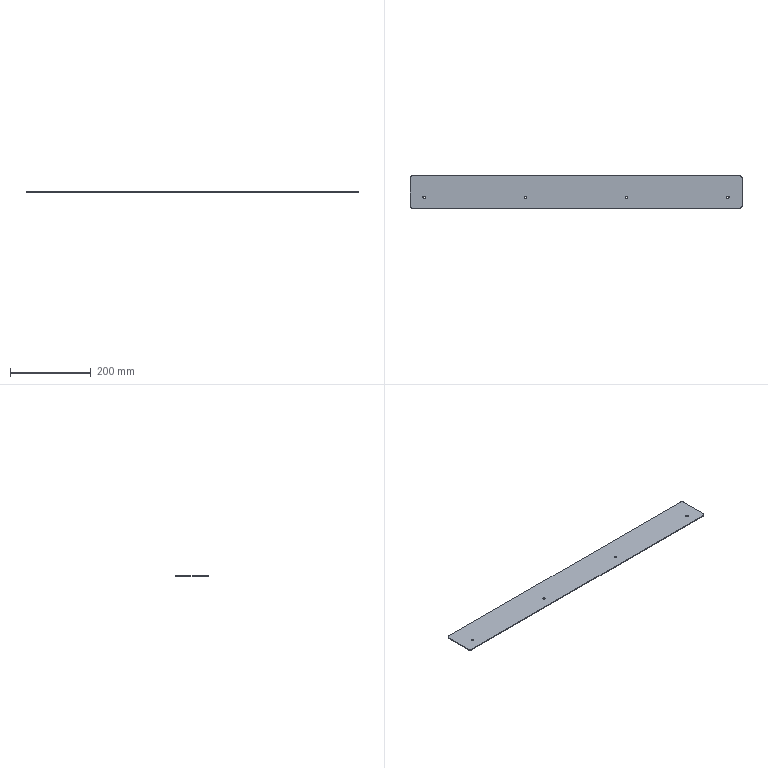Part | STEP file | 1 solid | 18 faces | box 820 x 80 x 2 mm | volume 130931 mm3 | cylinder 12 | plane 6 | commonest cylinder face diameters 6 x8 10 x4
STEP:
#1=CARTESIAN_POINT('',(0.,0.,0.));
#2=DIRECTION('',(0.,0.,1.));
#3=DIRECTION('',(1.,0.,0.));
#4=AXIS2_PLACEMENT_3D('',#1,#2,#3);
#5=CARTESIAN_POINT('',(-128.,-13.,2.));
#6=VERTEX_POINT('',#5);
#7=CARTESIAN_POINT('',(-128.,-13.,0.));
#8=VERTEX_POINT('',#7);
#9=CARTESIAN_POINT('',(-128.,-13.,0.));
#10=DIRECTION('',(0.,0.,-1.));
#11=VECTOR('',#10,1.);
#12=LINE('',#9,#11);
#13=CARTESIAN_POINT('',(-125.,-13.,0.));
#14=DIRECTION('',(0.,0.,-1.));
#15=DIRECTION('',(-1.,0.,0.));
#16=AXIS2_PLACEMENT_3D('',#13,#14,#15);
#17=CYLINDRICAL_SURFACE('',#16,3.);
#18=CARTESIAN_POINT('',(6.283,0.));
#19=DIRECTION('',(0.,1.));
#20=VECTOR('',#19,1.);
#21=LINE('',#18,#20);
#22=(GEOMETRIC_REPRESENTATION_CONTEXT(2)PARAMETRIC_REPRESENTATION_CONTEXT()REPRESENTATION_CONTEXT('',''));
#23=DEFINITIONAL_REPRESENTATION('',(#21),#22);
#24=PCURVE('',#17,#23);
#25=CARTESIAN_POINT('',(-125.,-13.,0.));
#26=DIRECTION('',(0.,0.,-1.));
#27=DIRECTION('',(-1.,0.,0.));
#28=AXIS2_PLACEMENT_3D('',#25,#26,#27);
#29=CYLINDRICAL_SURFACE('',#28,3.);
#30=CARTESIAN_POINT('',(0.,0.));
#31=DIRECTION('',(0.,1.));
#32=VECTOR('',#31,1.);
#33=LINE('',#30,#32);
#34=(GEOMETRIC_REPRESENTATION_CONTEXT(2)PARAMETRIC_REPRESENTATION_CONTEXT()REPRESENTATION_CONTEXT('',''));
#35=DEFINITIONAL_REPRESENTATION('',(#33),#34);
#36=PCURVE('',#29,#35);
#37=SURFACE_CURVE('',#12,(#24,#36),.PCURVE_S1.);
#38=EDGE_CURVE('',#6,#8,#37,.T.);
#39=ORIENTED_EDGE('',*,*,#38,.T.);
#40=CARTESIAN_POINT('',(-122.,-13.,0.));
#41=VERTEX_POINT('',#40);
#42=CARTESIAN_POINT('',(-125.,-13.,0.));
#43=DIRECTION('',(0.,0.,1.));
#44=DIRECTION('',(-1.,0.,0.));
#45=AXIS2_PLACEMENT_3D('',#42,#43,#44);
#46=CIRCLE('',#45,3.);
#47=CARTESIAN_POINT('',(6.283,0.));
#48=DIRECTION('',(-1.,0.));
#49=VECTOR('',#48,1.);
#50=LINE('',#47,#49);
#51=(GEOMETRIC_REPRESENTATION_CONTEXT(2)PARAMETRIC_REPRESENTATION_CONTEXT()REPRESENTATION_CONTEXT('',''));
#52=DEFINITIONAL_REPRESENTATION('',(#50),#51);
#53=PCURVE('',#17,#52);
#54=CARTESIAN_POINT('',(410.,-40.,0.));
#55=DIRECTION('',(0.,0.,1.));
#56=DIRECTION('',(1.,0.,0.));
#57=AXIS2_PLACEMENT_3D('',#54,#55,#56);
#58=PLANE('',#57);
#59=CARTESIAN_POINT('',(-535.,27.));
#60=DIRECTION('',(-1.,0.));
#61=AXIS2_PLACEMENT_2D('',#59,#60);
#62=CIRCLE('',#61,3.);
#63=(GEOMETRIC_REPRESENTATION_CONTEXT(2)PARAMETRIC_REPRESENTATION_CONTEXT()REPRESENTATION_CONTEXT('',''));
#64=DEFINITIONAL_REPRESENTATION('',(#62),#63);
#65=PCURVE('',#58,#64);
#66=SURFACE_CURVE('',#46,(#53,#65),.PCURVE_S1.);
#67=EDGE_CURVE('',#8,#41,#66,.T.);
#68=ORIENTED_EDGE('',*,*,#67,.T.);
#69=CARTESIAN_POINT('',(-122.,-13.,2.));
#70=VERTEX_POINT('',#69);
#71=CARTESIAN_POINT('',(-122.,-13.,0.));
#72=DIRECTION('',(0.,0.,-1.));
#73=VECTOR('',#72,1.);
#74=LINE('',#71,#73);
#75=CARTESIAN_POINT('',(3.142,0.));
#76=DIRECTION('',(0.,1.));
#77=VECTOR('',#76,1.);
#78=LINE('',#75,#77);
#79=(GEOMETRIC_REPRESENTATION_CONTEXT(2)PARAMETRIC_REPRESENTATION_CONTEXT()REPRESENTATION_CONTEXT('',''));
#80=DEFINITIONAL_REPRESENTATION('',(#78),#79);
#81=PCURVE('',#17,#80);
#82=CARTESIAN_POINT('',(3.142,0.));
#83=DIRECTION('',(0.,1.));
#84=VECTOR('',#83,1.);
#85=LINE('',#82,#84);
#86=(GEOMETRIC_REPRESENTATION_CONTEXT(2)PARAMETRIC_REPRESENTATION_CONTEXT()REPRESENTATION_CONTEXT('',''));
#87=DEFINITIONAL_REPRESENTATION('',(#85),#86);
#88=PCURVE('',#29,#87);
#89=SURFACE_CURVE('',#74,(#81,#88),.PCURVE_S1.);
#90=EDGE_CURVE('',#70,#41,#89,.T.);
#91=ORIENTED_EDGE('',*,*,#90,.F.);
#92=CARTESIAN_POINT('',(-125.,-13.,2.));
#93=DIRECTION('',(0.,0.,-1.));
#94=DIRECTION('',(-1.,0.,0.));
#95=AXIS2_PLACEMENT_3D('',#92,#93,#94);
#96=CIRCLE('',#95,3.);
#97=CARTESIAN_POINT('',(0.,-2.));
#98=DIRECTION('',(1.,0.));
#99=VECTOR('',#98,1.);
#100=LINE('',#97,#99);
#101=(GEOMETRIC_REPRESENTATION_CONTEXT(2)PARAMETRIC_REPRESENTATION_CONTEXT()REPRESENTATION_CONTEXT('',''));
#102=DEFINITIONAL_REPRESENTATION('',(#100),#101);
#103=PCURVE('',#17,#102);
#104=CARTESIAN_POINT('',(410.,-40.,2.));
#105=DIRECTION('',(0.,0.,1.));
#106=DIRECTION('',(1.,0.,0.));
#107=AXIS2_PLACEMENT_3D('',#104,#105,#106);
#108=PLANE('',#107);
#109=CARTESIAN_POINT('',(-538.,27.));
#110=CARTESIAN_POINT('',(-538.,32.196));
#111=CARTESIAN_POINT('',(-533.5,29.598));
#112=CARTESIAN_POINT('',(-529.,27.));
#113=CARTESIAN_POINT('',(-533.5,24.402));
#114=CARTESIAN_POINT('',(-538.,21.804));
#115=CARTESIAN_POINT('',(-538.,27.));
#116=(BOUNDED_CURVE()B_SPLINE_CURVE(2,(#109,#110,#111,#112,#113,#114,#115),.UNSPECIFIED.,.T.,.F.)B_SPLINE_CURVE_WITH_KNOTS((1,2,2,2,2,1),(-2.094,0.,2.094,4.189,6.283,8.378),.UNSPECIFIED.)CURVE()GEOMETRIC_REPRESENTATION_ITEM()RATIONAL_B_SPLINE_CURVE((1.,0.5,1.,0.5,1.,0.5,1.))REPRESENTATION_ITEM(''));
#117=(GEOMETRIC_REPRESENTATION_CONTEXT(2)PARAMETRIC_REPRESENTATION_CONTEXT()REPRESENTATION_CONTEXT('',''));
#118=DEFINITIONAL_REPRESENTATION('',(#116),#117);
#119=PCURVE('',#108,#118);
#120=SURFACE_CURVE('',#96,(#103,#119),.PCURVE_S1.);
#121=EDGE_CURVE('',#70,#6,#120,.T.);
#122=ORIENTED_EDGE('',*,*,#121,.T.);
#123=EDGE_LOOP('',(#39,#68,#91,#122));
#124=FACE_BOUND('',#123,.F.);
#125=ADVANCED_FACE('',(#124),#17,.F.);
#126=CARTESIAN_POINT('',(-378.,-13.,2.));
#127=VERTEX_POINT('',#126);
#128=CARTESIAN_POINT('',(-378.,-13.,0.));
#129=VERTEX_POINT('',#128);
#130=CARTESIAN_POINT('',(-378.,-13.,0.));
#131=DIRECTION('',(0.,0.,-1.));
#132=VECTOR('',#131,1.);
#133=LINE('',#130,#132);
#134=CARTESIAN_POINT('',(-375.,-13.,0.));
#135=DIRECTION('',(0.,0.,-1.));
#136=DIRECTION('',(-1.,0.,0.));
#137=AXIS2_PLACEMENT_3D('',#134,#135,#136);
#138=CYLINDRICAL_SURFACE('',#137,3.);
#139=CARTESIAN_POINT('',(6.283,0.));
#140=DIRECTION('',(0.,1.));
#141=VECTOR('',#140,1.);
#142=LINE('',#139,#141);
#143=(GEOMETRIC_REPRESENTATION_CONTEXT(2)PARAMETRIC_REPRESENTATION_CONTEXT()REPRESENTATION_CONTEXT('',''));
#144=DEFINITIONAL_REPRESENTATION('',(#142),#143);
#145=PCURVE('',#138,#144);
#146=CARTESIAN_POINT('',(-375.,-13.,0.));
#147=DIRECTION('',(0.,0.,-1.));
#148=DIRECTION('',(-1.,0.,0.));
#149=AXIS2_PLACEMENT_3D('',#146,#147,#148);
#150=CYLINDRICAL_SURFACE('',#149,3.);
#151=CARTESIAN_POINT('',(0.,0.));
#152=DIRECTION('',(0.,1.));
#153=VECTOR('',#152,1.);
#154=LINE('',#151,#153);
#155=(GEOMETRIC_REPRESENTATION_CONTEXT(2)PARAMETRIC_REPRESENTATION_CONTEXT()REPRESENTATION_CONTEXT('',''));
#156=DEFINITIONAL_REPRESENTATION('',(#154),#155);
#157=PCURVE('',#150,#156);
#158=SURFACE_CURVE('',#133,(#145,#157),.PCURVE_S1.);
#159=EDGE_CURVE('',#127,#129,#158,.T.);
#160=ORIENTED_EDGE('',*,*,#159,.T.);
#161=CARTESIAN_POINT('',(-372.,-13.,0.));
#162=VERTEX_POINT('',#161);
#163=CARTESIAN_POINT('',(-375.,-13.,0.));
#164=DIRECTION('',(0.,0.,1.));
#165=DIRECTION('',(-1.,0.,0.));
#166=AXIS2_PLACEMENT_3D('',#163,#164,#165);
#167=CIRCLE('',#166,3.);
#168=CARTESIAN_POINT('',(6.283,0.));
#169=DIRECTION('',(-1.,0.));
#170=VECTOR('',#169,1.);
#171=LINE('',#168,#170);
#172=(GEOMETRIC_REPRESENTATION_CONTEXT(2)PARAMETRIC_REPRESENTATION_CONTEXT()REPRESENTATION_CONTEXT('',''));
#173=DEFINITIONAL_REPRESENTATION('',(#171),#172);
#174=PCURVE('',#138,#173);
#175=CARTESIAN_POINT('',(-785.,27.));
#176=DIRECTION('',(-1.,0.));
#177=AXIS2_PLACEMENT_2D('',#175,#176);
#178=CIRCLE('',#177,3.);
#179=(GEOMETRIC_REPRESENTATION_CONTEXT(2)PARAMETRIC_REPRESENTATION_CONTEXT()REPRESENTATION_CONTEXT('',''));
#180=DEFINITIONAL_REPRESENTATION('',(#178),#179);
#181=PCURVE('',#58,#180);
#182=SURFACE_CURVE('',#167,(#174,#181),.PCURVE_S1.);
#183=EDGE_CURVE('',#129,#162,#182,.T.);
#184=ORIENTED_EDGE('',*,*,#183,.T.);
#185=CARTESIAN_POINT('',(-372.,-13.,2.));
#186=VERTEX_POINT('',#185);
#187=CARTESIAN_POINT('',(-372.,-13.,0.));
#188=DIRECTION('',(0.,0.,-1.));
#189=VECTOR('',#188,1.);
#190=LINE('',#187,#189);
#191=CARTESIAN_POINT('',(3.142,0.));
#192=DIRECTION('',(0.,1.));
#193=VECTOR('',#192,1.);
#194=LINE('',#191,#193);
#195=(GEOMETRIC_REPRESENTATION_CONTEXT(2)PARAMETRIC_REPRESENTATION_CONTEXT()REPRESENTATION_CONTEXT('',''));
#196=DEFINITIONAL_REPRESENTATION('',(#194),#195);
#197=PCURVE('',#138,#196);
#198=CARTESIAN_POINT('',(3.142,0.));
#199=DIRECTION('',(0.,1.));
#200=VECTOR('',#199,1.);
#201=LINE('',#198,#200);
#202=(GEOMETRIC_REPRESENTATION_CONTEXT(2)PARAMETRIC_REPRESENTATION_CONTEXT()REPRESENTATION_CONTEXT('',''));
#203=DEFINITIONAL_REPRESENTATION('',(#201),#202);
#204=PCURVE('',#150,#203);
#205=SURFACE_CURVE('',#190,(#197,#204),.PCURVE_S1.);
#206=EDGE_CURVE('',#186,#162,#205,.T.);
#207=ORIENTED_EDGE('',*,*,#206,.F.);
#208=CARTESIAN_POINT('',(-375.,-13.,2.));
#209=DIRECTION('',(0.,0.,-1.));
#210=DIRECTION('',(-1.,0.,0.));
#211=AXIS2_PLACEMENT_3D('',#208,#209,#210);
#212=CIRCLE('',#211,3.);
#213=CARTESIAN_POINT('',(0.,-2.));
#214=DIRECTION('',(1.,0.));
#215=VECTOR('',#214,1.);
#216=LINE('',#213,#215);
#217=(GEOMETRIC_REPRESENTATION_CONTEXT(2)PARAMETRIC_REPRESENTATION_CONTEXT()REPRESENTATION_CONTEXT('',''));
#218=DEFINITIONAL_REPRESENTATION('',(#216),#217);
#219=PCURVE('',#138,#218);
#220=CARTESIAN_POINT('',(-788.,27.));
#221=CARTESIAN_POINT('',(-788.,32.196));
#222=CARTESIAN_POINT('',(-783.5,29.598));
#223=CARTESIAN_POINT('',(-779.,27.));
#224=CARTESIAN_POINT('',(-783.5,24.402));
#225=CARTESIAN_POINT('',(-788.,21.804));
#226=CARTESIAN_POINT('',(-788.,27.));
#227=(BOUNDED_CURVE()B_SPLINE_CURVE(2,(#220,#221,#222,#223,#224,#225,#226),.UNSPECIFIED.,.T.,.F.)B_SPLINE_CURVE_WITH_KNOTS((1,2,2,2,2,1),(-2.094,0.,2.094,4.189,6.283,8.378),.UNSPECIFIED.)CURVE()GEOMETRIC_REPRESENTATION_ITEM()RATIONAL_B_SPLINE_CURVE((1.,0.5,1.,0.5,1.,0.5,1.))REPRESENTATION_ITEM(''));
#228=(GEOMETRIC_REPRESENTATION_CONTEXT(2)PARAMETRIC_REPRESENTATION_CONTEXT()REPRESENTATION_CONTEXT('',''));
#229=DEFINITIONAL_REPRESENTATION('',(#227),#228);
#230=PCURVE('',#108,#229);
#231=SURFACE_CURVE('',#212,(#219,#230),.PCURVE_S1.);
#232=EDGE_CURVE('',#186,#127,#231,.T.);
#233=ORIENTED_EDGE('',*,*,#232,.T.);
#234=EDGE_LOOP('',(#160,#184,#207,#233));
#235=FACE_BOUND('',#234,.F.);
#236=ADVANCED_FACE('',(#235),#138,.F.);
#237=CARTESIAN_POINT('',(122.,-13.,2.));
#238=VERTEX_POINT('',#237);
#239=CARTESIAN_POINT('',(122.,-13.,0.));
#240=VERTEX_POINT('',#239);
#241=CARTESIAN_POINT('',(122.,-13.,0.));
#242=DIRECTION('',(0.,0.,-1.));
#243=VECTOR('',#242,1.);
#244=LINE('',#241,#243);
#245=CARTESIAN_POINT('',(125.,-13.,0.));
#246=DIRECTION('',(0.,0.,-1.));
#247=DIRECTION('',(-1.,0.,0.));
#248=AXIS2_PLACEMENT_3D('',#245,#246,#247);
#249=CYLINDRICAL_SURFACE('',#248,3.);
#250=CARTESIAN_POINT('',(6.283,0.));
#251=DIRECTION('',(0.,1.));
#252=VECTOR('',#251,1.);
#253=LINE('',#250,#252);
#254=(GEOMETRIC_REPRESENTATION_CONTEXT(2)PARAMETRIC_REPRESENTATION_CONTEXT()REPRESENTATION_CONTEXT('',''));
#255=DEFINITIONAL_REPRESENTATION('',(#253),#254);
#256=PCURVE('',#249,#255);
#257=CARTESIAN_POINT('',(125.,-13.,0.));
#258=DIRECTION('',(0.,0.,-1.));
#259=DIRECTION('',(-1.,0.,0.));
#260=AXIS2_PLACEMENT_3D('',#257,#258,#259);
#261=CYLINDRICAL_SURFACE('',#260,3.);
#262=CARTESIAN_POINT('',(0.,0.));
#263=DIRECTION('',(0.,1.));
#264=VECTOR('',#263,1.);
#265=LINE('',#262,#264);
#266=(GEOMETRIC_REPRESENTATION_CONTEXT(2)PARAMETRIC_REPRESENTATION_CONTEXT()REPRESENTATION_CONTEXT('',''));
#267=DEFINITIONAL_REPRESENTATION('',(#265),#266);
#268=PCURVE('',#261,#267);
#269=SURFACE_CURVE('',#244,(#256,#268),.PCURVE_S1.);
#270=EDGE_CURVE('',#238,#240,#269,.T.);
#271=ORIENTED_EDGE('',*,*,#270,.T.);
#272=CARTESIAN_POINT('',(128.,-13.,0.));
#273=VERTEX_POINT('',#272);
#274=CARTESIAN_POINT('',(125.,-13.,0.));
#275=DIRECTION('',(0.,0.,1.));
#276=DIRECTION('',(-1.,0.,0.));
#277=AXIS2_PLACEMENT_3D('',#274,#275,#276);
#278=CIRCLE('',#277,3.);
#279=CARTESIAN_POINT('',(6.283,0.));
#280=DIRECTION('',(-1.,0.));
#281=VECTOR('',#280,1.);
#282=LINE('',#279,#281);
#283=(GEOMETRIC_REPRESENTATION_CONTEXT(2)PARAMETRIC_REPRESENTATION_CONTEXT()REPRESENTATION_CONTEXT('',''));
#284=DEFINITIONAL_REPRESENTATION('',(#282),#283);
#285=PCURVE('',#249,#284);
#286=CARTESIAN_POINT('',(-285.,27.));
#287=DIRECTION('',(-1.,0.));
#288=AXIS2_PLACEMENT_2D('',#286,#287);
#289=CIRCLE('',#288,3.);
#290=(GEOMETRIC_REPRESENTATION_CONTEXT(2)PARAMETRIC_REPRESENTATION_CONTEXT()REPRESENTATION_CONTEXT('',''));
#291=DEFINITIONAL_REPRESENTATION('',(#289),#290);
#292=PCURVE('',#58,#291);
#293=SURFACE_CURVE('',#278,(#285,#292),.PCURVE_S1.);
#294=EDGE_CURVE('',#240,#273,#293,.T.);
#295=ORIENTED_EDGE('',*,*,#294,.T.);
#296=CARTESIAN_POINT('',(128.,-13.,2.));
#297=VERTEX_POINT('',#296);
#298=CARTESIAN_POINT('',(128.,-13.,0.));
#299=DIRECTION('',(0.,0.,-1.));
#300=VECTOR('',#299,1.);
#301=LINE('',#298,#300);
#302=CARTESIAN_POINT('',(3.142,0.));
#303=DIRECTION('',(0.,1.));
#304=VECTOR('',#303,1.);
#305=LINE('',#302,#304);
#306=(GEOMETRIC_REPRESENTATION_CONTEXT(2)PARAMETRIC_REPRESENTATION_CONTEXT()REPRESENTATION_CONTEXT('',''));
#307=DEFINITIONAL_REPRESENTATION('',(#305),#306);
#308=PCURVE('',#249,#307);
#309=CARTESIAN_POINT('',(3.142,0.));
#310=DIRECTION('',(0.,1.));
#311=VECTOR('',#310,1.);
#312=LINE('',#309,#311);
#313=(GEOMETRIC_REPRESENTATION_CONTEXT(2)PARAMETRIC_REPRESENTATION_CONTEXT()REPRESENTATION_CONTEXT('',''));
#314=DEFINITIONAL_REPRESENTATION('',(#312),#313);
#315=PCURVE('',#261,#314);
#316=SURFACE_CURVE('',#301,(#308,#315),.PCURVE_S1.);
#317=EDGE_CURVE('',#297,#273,#316,.T.);
#318=ORIENTED_EDGE('',*,*,#317,.F.);
#319=CARTESIAN_POINT('',(125.,-13.,2.));
#320=DIRECTION('',(0.,0.,-1.));
#321=DIRECTION('',(-1.,0.,0.));
#322=AXIS2_PLACEMENT_3D('',#319,#320,#321);
#323=CIRCLE('',#322,3.);
#324=CARTESIAN_POINT('',(0.,-2.));
#325=DIRECTION('',(1.,0.));
#326=VECTOR('',#325,1.);
#327=LINE('',#324,#326);
#328=(GEOMETRIC_REPRESENTATION_CONTEXT(2)PARAMETRIC_REPRESENTATION_CONTEXT()REPRESENTATION_CONTEXT('',''));
#329=DEFINITIONAL_REPRESENTATION('',(#327),#328);
#330=PCURVE('',#249,#329);
#331=CARTESIAN_POINT('',(-288.,27.));
#332=CARTESIAN_POINT('',(-288.,32.196));
#333=CARTESIAN_POINT('',(-283.5,29.598));
#334=CARTESIAN_POINT('',(-279.,27.));
#335=CARTESIAN_POINT('',(-283.5,24.402));
#336=CARTESIAN_POINT('',(-288.,21.804));
#337=CARTESIAN_POINT('',(-288.,27.));
#338=(BOUNDED_CURVE()B_SPLINE_CURVE(2,(#331,#332,#333,#334,#335,#336,#337),.UNSPECIFIED.,.T.,.F.)B_SPLINE_CURVE_WITH_KNOTS((1,2,2,2,2,1),(-2.094,0.,2.094,4.189,6.283,8.378),.UNSPECIFIED.)CURVE()GEOMETRIC_REPRESENTATION_ITEM()RATIONAL_B_SPLINE_CURVE((1.,0.5,1.,0.5,1.,0.5,1.))REPRESENTATION_ITEM(''));
#339=(GEOMETRIC_REPRESENTATION_CONTEXT(2)PARAMETRIC_REPRESENTATION_CONTEXT()REPRESENTATION_CONTEXT('',''));
#340=DEFINITIONAL_REPRESENTATION('',(#338),#339);
#341=PCURVE('',#108,#340);
#342=SURFACE_CURVE('',#323,(#330,#341),.PCURVE_S1.);
#343=EDGE_CURVE('',#297,#238,#342,.T.);
#344=ORIENTED_EDGE('',*,*,#343,.T.);
#345=EDGE_LOOP('',(#271,#295,#318,#344));
#346=FACE_BOUND('',#345,.F.);
#347=ADVANCED_FACE('',(#346),#249,.F.);
#348=CARTESIAN_POINT('',(372.,-13.,2.));
#349=VERTEX_POINT('',#348);
#350=CARTESIAN_POINT('',(372.,-13.,0.));
#351=VERTEX_POINT('',#350);
#352=CARTESIAN_POINT('',(372.,-13.,0.));
#353=DIRECTION('',(0.,0.,-1.));
#354=VECTOR('',#353,1.);
#355=LINE('',#352,#354);
#356=CARTESIAN_POINT('',(375.,-13.,0.));
#357=DIRECTION('',(0.,0.,-1.));
#358=DIRECTION('',(-1.,0.,0.));
#359=AXIS2_PLACEMENT_3D('',#356,#357,#358);
#360=CYLINDRICAL_SURFACE('',#359,3.);
#361=CARTESIAN_POINT('',(6.283,0.));
#362=DIRECTION('',(0.,1.));
#363=VECTOR('',#362,1.);
#364=LINE('',#361,#363);
#365=(GEOMETRIC_REPRESENTATION_CONTEXT(2)PARAMETRIC_REPRESENTATION_CONTEXT()REPRESENTATION_CONTEXT('',''));
#366=DEFINITIONAL_REPRESENTATION('',(#364),#365);
#367=PCURVE('',#360,#366);
#368=CARTESIAN_POINT('',(375.,-13.,0.));
#369=DIRECTION('',(0.,0.,-1.));
#370=DIRECTION('',(-1.,0.,0.));
#371=AXIS2_PLACEMENT_3D('',#368,#369,#370);
#372=CYLINDRICAL_SURFACE('',#371,3.);
#373=CARTESIAN_POINT('',(0.,0.));
#374=DIRECTION('',(0.,1.));
#375=VECTOR('',#374,1.);
#376=LINE('',#373,#375);
#377=(GEOMETRIC_REPRESENTATION_CONTEXT(2)PARAMETRIC_REPRESENTATION_CONTEXT()REPRESENTATION_CONTEXT('',''));
#378=DEFINITIONAL_REPRESENTATION('',(#376),#377);
#379=PCURVE('',#372,#378);
#380=SURFACE_CURVE('',#355,(#367,#379),.PCURVE_S1.);
#381=EDGE_CURVE('',#349,#351,#380,.T.);
#382=ORIENTED_EDGE('',*,*,#381,.T.);
#383=CARTESIAN_POINT('',(378.,-13.,0.));
#384=VERTEX_POINT('',#383);
#385=CARTESIAN_POINT('',(375.,-13.,0.));
#386=DIRECTION('',(0.,0.,1.));
#387=DIRECTION('',(-1.,0.,0.));
#388=AXIS2_PLACEMENT_3D('',#385,#386,#387);
#389=CIRCLE('',#388,3.);
#390=CARTESIAN_POINT('',(6.283,0.));
#391=DIRECTION('',(-1.,0.));
#392=VECTOR('',#391,1.);
#393=LINE('',#390,#392);
#394=(GEOMETRIC_REPRESENTATION_CONTEXT(2)PARAMETRIC_REPRESENTATION_CONTEXT()REPRESENTATION_CONTEXT('',''));
#395=DEFINITIONAL_REPRESENTATION('',(#393),#394);
#396=PCURVE('',#360,#395);
#397=CARTESIAN_POINT('',(-35.,27.));
#398=DIRECTION('',(-1.,0.));
#399=AXIS2_PLACEMENT_2D('',#397,#398);
#400=CIRCLE('',#399,3.);
#401=(GEOMETRIC_REPRESENTATION_CONTEXT(2)PARAMETRIC_REPRESENTATION_CONTEXT()REPRESENTATION_CONTEXT('',''));
#402=DEFINITIONAL_REPRESENTATION('',(#400),#401);
#403=PCURVE('',#58,#402);
#404=SURFACE_CURVE('',#389,(#396,#403),.PCURVE_S1.);
#405=EDGE_CURVE('',#351,#384,#404,.T.);
#406=ORIENTED_EDGE('',*,*,#405,.T.);
#407=CARTESIAN_POINT('',(378.,-13.,2.));
#408=VERTEX_POINT('',#407);
#409=CARTESIAN_POINT('',(378.,-13.,0.));
#410=DIRECTION('',(0.,0.,-1.));
#411=VECTOR('',#410,1.);
#412=LINE('',#409,#411);
#413=CARTESIAN_POINT('',(3.142,0.));
#414=DIRECTION('',(0.,1.));
#415=VECTOR('',#414,1.);
#416=LINE('',#413,#415);
#417=(GEOMETRIC_REPRESENTATION_CONTEXT(2)PARAMETRIC_REPRESENTATION_CONTEXT()REPRESENTATION_CONTEXT('',''));
#418=DEFINITIONAL_REPRESENTATION('',(#416),#417);
#419=PCURVE('',#360,#418);
#420=CARTESIAN_POINT('',(3.142,0.));
#421=DIRECTION('',(0.,1.));
#422=VECTOR('',#421,1.);
#423=LINE('',#420,#422);
#424=(GEOMETRIC_REPRESENTATION_CONTEXT(2)PARAMETRIC_REPRESENTATION_CONTEXT()REPRESENTATION_CONTEXT('',''));
#425=DEFINITIONAL_REPRESENTATION('',(#423),#424);
#426=PCURVE('',#372,#425);
#427=SURFACE_CURVE('',#412,(#419,#426),.PCURVE_S1.);
#428=EDGE_CURVE('',#408,#384,#427,.T.);
#429=ORIENTED_EDGE('',*,*,#428,.F.);
#430=CARTESIAN_POINT('',(375.,-13.,2.));
#431=DIRECTION('',(0.,0.,-1.));
#432=DIRECTION('',(-1.,0.,0.));
#433=AXIS2_PLACEMENT_3D('',#430,#431,#432);
#434=CIRCLE('',#433,3.);
#435=CARTESIAN_POINT('',(0.,-2.));
#436=DIRECTION('',(1.,0.));
#437=VECTOR('',#436,1.);
#438=LINE('',#435,#437);
#439=(GEOMETRIC_REPRESENTATION_CONTEXT(2)PARAMETRIC_REPRESENTATION_CONTEXT()REPRESENTATION_CONTEXT('',''));
#440=DEFINITIONAL_REPRESENTATION('',(#438),#439);
#441=PCURVE('',#360,#440);
#442=CARTESIAN_POINT('',(-38.,27.));
#443=CARTESIAN_POINT('',(-38.,32.196));
#444=CARTESIAN_POINT('',(-33.5,29.598));
#445=CARTESIAN_POINT('',(-29.,27.));
#446=CARTESIAN_POINT('',(-33.5,24.402));
#447=CARTESIAN_POINT('',(-38.,21.804));
#448=CARTESIAN_POINT('',(-38.,27.));
#449=(BOUNDED_CURVE()B_SPLINE_CURVE(2,(#442,#443,#444,#445,#446,#447,#448),.UNSPECIFIED.,.T.,.F.)B_SPLINE_CURVE_WITH_KNOTS((1,2,2,2,2,1),(-2.094,0.,2.094,4.189,6.283,8.378),.UNSPECIFIED.)CURVE()GEOMETRIC_REPRESENTATION_ITEM()RATIONAL_B_SPLINE_CURVE((1.,0.5,1.,0.5,1.,0.5,1.))REPRESENTATION_ITEM(''));
#450=(GEOMETRIC_REPRESENTATION_CONTEXT(2)PARAMETRIC_REPRESENTATION_CONTEXT()REPRESENTATION_CONTEXT('',''));
#451=DEFINITIONAL_REPRESENTATION('',(#449),#450);
#452=PCURVE('',#108,#451);
#453=SURFACE_CURVE('',#434,(#441,#452),.PCURVE_S1.);
#454=EDGE_CURVE('',#408,#349,#453,.T.);
#455=ORIENTED_EDGE('',*,*,#454,.T.);
#456=EDGE_LOOP('',(#382,#406,#429,#455));
#457=FACE_BOUND('',#456,.F.);
#458=ADVANCED_FACE('',(#457),#360,.F.);
#459=CARTESIAN_POINT('',(-125.,-13.,2.));
#460=DIRECTION('',(0.,0.,-1.));
#461=DIRECTION('',(-1.,0.,0.));
#462=AXIS2_PLACEMENT_3D('',#459,#460,#461);
#463=CIRCLE('',#462,3.);
#464=CARTESIAN_POINT('',(-538.,27.));
#465=CARTESIAN_POINT('',(-538.,32.196));
#466=CARTESIAN_POINT('',(-533.5,29.598));
#467=CARTESIAN_POINT('',(-529.,27.));
#468=CARTESIAN_POINT('',(-533.5,24.402));
#469=CARTESIAN_POINT('',(-538.,21.804));
#470=CARTESIAN_POINT('',(-538.,27.));
#471=(BOUNDED_CURVE()B_SPLINE_CURVE(2,(#464,#465,#466,#467,#468,#469,#470),.UNSPECIFIED.,.T.,.F.)B_SPLINE_CURVE_WITH_KNOTS((1,2,2,2,2,1),(-2.094,0.,2.094,4.189,6.283,8.378),.UNSPECIFIED.)CURVE()GEOMETRIC_REPRESENTATION_ITEM()RATIONAL_B_SPLINE_CURVE((1.,0.5,1.,0.5,1.,0.5,1.))REPRESENTATION_ITEM(''));
#472=(GEOMETRIC_REPRESENTATION_CONTEXT(2)PARAMETRIC_REPRESENTATION_CONTEXT()REPRESENTATION_CONTEXT('',''));
#473=DEFINITIONAL_REPRESENTATION('',(#471),#472);
#474=PCURVE('',#108,#473);
#475=CARTESIAN_POINT('',(0.,-2.));
#476=DIRECTION('',(1.,0.));
#477=VECTOR('',#476,1.);
#478=LINE('',#475,#477);
#479=(GEOMETRIC_REPRESENTATION_CONTEXT(2)PARAMETRIC_REPRESENTATION_CONTEXT()REPRESENTATION_CONTEXT('',''));
#480=DEFINITIONAL_REPRESENTATION('',(#478),#479);
#481=PCURVE('',#29,#480);
#482=SURFACE_CURVE('',#463,(#474,#481),.PCURVE_S1.);
#483=EDGE_CURVE('',#6,#70,#482,.T.);
#484=ORIENTED_EDGE('',*,*,#483,.T.);
#485=ORIENTED_EDGE('',*,*,#121,.T.);
#486=EDGE_LOOP('',(#484,#485));
#487=FACE_BOUND('',#486,.T.);
#488=CARTESIAN_POINT('',(-375.,-13.,2.));
#489=DIRECTION('',(0.,0.,-1.));
#490=DIRECTION('',(-1.,0.,0.));
#491=AXIS2_PLACEMENT_3D('',#488,#489,#490);
#492=CIRCLE('',#491,3.);
#493=CARTESIAN_POINT('',(-788.,27.));
#494=CARTESIAN_POINT('',(-788.,32.196));
#495=CARTESIAN_POINT('',(-783.5,29.598));
#496=CARTESIAN_POINT('',(-779.,27.));
#497=CARTESIAN_POINT('',(-783.5,24.402));
#498=CARTESIAN_POINT('',(-788.,21.804));
#499=CARTESIAN_POINT('',(-788.,27.));
#500=(BOUNDED_CURVE()B_SPLINE_CURVE(2,(#493,#494,#495,#496,#497,#498,#499),.UNSPECIFIED.,.T.,.F.)B_SPLINE_CURVE_WITH_KNOTS((1,2,2,2,2,1),(-2.094,0.,2.094,4.189,6.283,8.378),.UNSPECIFIED.)CURVE()GEOMETRIC_REPRESENTATION_ITEM()RATIONAL_B_SPLINE_CURVE((1.,0.5,1.,0.5,1.,0.5,1.))REPRESENTATION_ITEM(''));
#501=(GEOMETRIC_REPRESENTATION_CONTEXT(2)PARAMETRIC_REPRESENTATION_CONTEXT()REPRESENTATION_CONTEXT('',''));
#502=DEFINITIONAL_REPRESENTATION('',(#500),#501);
#503=PCURVE('',#108,#502);
#504=CARTESIAN_POINT('',(0.,-2.));
#505=DIRECTION('',(1.,0.));
#506=VECTOR('',#505,1.);
#507=LINE('',#504,#506);
#508=(GEOMETRIC_REPRESENTATION_CONTEXT(2)PARAMETRIC_REPRESENTATION_CONTEXT()REPRESENTATION_CONTEXT('',''));
#509=DEFINITIONAL_REPRESENTATION('',(#507),#508);
#510=PCURVE('',#150,#509);
#511=SURFACE_CURVE('',#492,(#503,#510),.PCURVE_S1.);
#512=EDGE_CURVE('',#127,#186,#511,.T.);
#513=ORIENTED_EDGE('',*,*,#512,.T.);
#514=ORIENTED_EDGE('',*,*,#232,.T.);
#515=EDGE_LOOP('',(#513,#514));
#516=FACE_BOUND('',#515,.T.);
#517=CARTESIAN_POINT('',(125.,-13.,2.));
#518=DIRECTION('',(0.,0.,-1.));
#519=DIRECTION('',(-1.,0.,0.));
#520=AXIS2_PLACEMENT_3D('',#517,#518,#519);
#521=CIRCLE('',#520,3.);
#522=CARTESIAN_POINT('',(-288.,27.));
#523=CARTESIAN_POINT('',(-288.,32.196));
#524=CARTESIAN_POINT('',(-283.5,29.598));
#525=CARTESIAN_POINT('',(-279.,27.));
#526=CARTESIAN_POINT('',(-283.5,24.402));
#527=CARTESIAN_POINT('',(-288.,21.804));
#528=CARTESIAN_POINT('',(-288.,27.));
#529=(BOUNDED_CURVE()B_SPLINE_CURVE(2,(#522,#523,#524,#525,#526,#527,#528),.UNSPECIFIED.,.T.,.F.)B_SPLINE_CURVE_WITH_KNOTS((1,2,2,2,2,1),(-2.094,0.,2.094,4.189,6.283,8.378),.UNSPECIFIED.)CURVE()GEOMETRIC_REPRESENTATION_ITEM()RATIONAL_B_SPLINE_CURVE((1.,0.5,1.,0.5,1.,0.5,1.))REPRESENTATION_ITEM(''));
#530=(GEOMETRIC_REPRESENTATION_CONTEXT(2)PARAMETRIC_REPRESENTATION_CONTEXT()REPRESENTATION_CONTEXT('',''));
#531=DEFINITIONAL_REPRESENTATION('',(#529),#530);
#532=PCURVE('',#108,#531);
#533=CARTESIAN_POINT('',(0.,-2.));
#534=DIRECTION('',(1.,0.));
#535=VECTOR('',#534,1.);
#536=LINE('',#533,#535);
#537=(GEOMETRIC_REPRESENTATION_CONTEXT(2)PARAMETRIC_REPRESENTATION_CONTEXT()REPRESENTATION_CONTEXT('',''));
#538=DEFINITIONAL_REPRESENTATION('',(#536),#537);
#539=PCURVE('',#261,#538);
#540=SURFACE_CURVE('',#521,(#532,#539),.PCURVE_S1.);
#541=EDGE_CURVE('',#238,#297,#540,.T.);
#542=ORIENTED_EDGE('',*,*,#541,.T.);
#543=ORIENTED_EDGE('',*,*,#343,.T.);
#544=EDGE_LOOP('',(#542,#543));
#545=FACE_BOUND('',#544,.T.);
#546=CARTESIAN_POINT('',(375.,-13.,2.));
#547=DIRECTION('',(0.,0.,-1.));
#548=DIRECTION('',(-1.,0.,0.));
#549=AXIS2_PLACEMENT_3D('',#546,#547,#548);
#550=CIRCLE('',#549,3.);
#551=CARTESIAN_POINT('',(-38.,27.));
#552=CARTESIAN_POINT('',(-38.,32.196));
#553=CARTESIAN_POINT('',(-33.5,29.598));
#554=CARTESIAN_POINT('',(-29.,27.));
#555=CARTESIAN_POINT('',(-33.5,24.402));
#556=CARTESIAN_POINT('',(-38.,21.804));
#557=CARTESIAN_POINT('',(-38.,27.));
#558=(BOUNDED_CURVE()B_SPLINE_CURVE(2,(#551,#552,#553,#554,#555,#556,#557),.UNSPECIFIED.,.T.,.F.)B_SPLINE_CURVE_WITH_KNOTS((1,2,2,2,2,1),(-2.094,0.,2.094,4.189,6.283,8.378),.UNSPECIFIED.)CURVE()GEOMETRIC_REPRESENTATION_ITEM()RATIONAL_B_SPLINE_CURVE((1.,0.5,1.,0.5,1.,0.5,1.))REPRESENTATION_ITEM(''));
#559=(GEOMETRIC_REPRESENTATION_CONTEXT(2)PARAMETRIC_REPRESENTATION_CONTEXT()REPRESENTATION_CONTEXT('',''));
#560=DEFINITIONAL_REPRESENTATION('',(#558),#559);
#561=PCURVE('',#108,#560);
#562=CARTESIAN_POINT('',(0.,-2.));
#563=DIRECTION('',(1.,0.));
#564=VECTOR('',#563,1.);
#565=LINE('',#562,#564);
#566=(GEOMETRIC_REPRESENTATION_CONTEXT(2)PARAMETRIC_REPRESENTATION_CONTEXT()REPRESENTATION_CONTEXT('',''));
#567=DEFINITIONAL_REPRESENTATION('',(#565),#566);
#568=PCURVE('',#372,#567);
#569=SURFACE_CURVE('',#550,(#561,#568),.PCURVE_S1.);
#570=EDGE_CURVE('',#349,#408,#569,.T.);
#571=ORIENTED_EDGE('',*,*,#570,.T.);
#572=ORIENTED_EDGE('',*,*,#454,.T.);
#573=EDGE_LOOP('',(#571,#572));
#574=FACE_BOUND('',#573,.T.);
#575=CARTESIAN_POINT('',(405.,40.,2.));
#576=VERTEX_POINT('',#575);
#577=CARTESIAN_POINT('',(-405.,40.,2.));
#578=VERTEX_POINT('',#577);
#579=CARTESIAN_POINT('',(410.,40.,2.));
#580=DIRECTION('',(-1.,0.,0.));
#581=VECTOR('',#580,1.);
#582=LINE('',#579,#581);
#583=CARTESIAN_POINT('',(0.,80.));
#584=DIRECTION('',(-1.,0.));
#585=VECTOR('',#584,1.);
#586=LINE('',#583,#585);
#587=(GEOMETRIC_REPRESENTATION_CONTEXT(2)PARAMETRIC_REPRESENTATION_CONTEXT()REPRESENTATION_CONTEXT('',''));
#588=DEFINITIONAL_REPRESENTATION('',(#586),#587);
#589=PCURVE('',#108,#588);
#590=CARTESIAN_POINT('',(-410.,40.,2.));
#591=DIRECTION('',(0.,-1.,0.));
#592=DIRECTION('',(0.,0.,-1.));
#593=AXIS2_PLACEMENT_3D('',#590,#591,#592);
#594=PLANE('',#593);
#595=CARTESIAN_POINT('',(0.,820.));
#596=DIRECTION('',(0.,-1.));
#597=VECTOR('',#596,1.);
#598=LINE('',#595,#597);
#599=(GEOMETRIC_REPRESENTATION_CONTEXT(2)PARAMETRIC_REPRESENTATION_CONTEXT()REPRESENTATION_CONTEXT('',''));
#600=DEFINITIONAL_REPRESENTATION('',(#598),#599);
#601=PCURVE('',#594,#600);
#602=SURFACE_CURVE('',#582,(#589,#601),.PCURVE_S1.);
#603=EDGE_CURVE('',#576,#578,#602,.T.);
#604=ORIENTED_EDGE('',*,*,#603,.T.);
#605=CARTESIAN_POINT('',(-410.,35.,2.));
#606=VERTEX_POINT('',#605);
#607=CARTESIAN_POINT('',(-405.,35.,2.));
#608=DIRECTION('',(0.,0.,1.));
#609=DIRECTION('',(1.,0.,0.));
#610=AXIS2_PLACEMENT_3D('',#607,#608,#609);
#611=CIRCLE('',#610,5.);
#612=CARTESIAN_POINT('',(-815.,75.));
#613=DIRECTION('',(1.,0.));
#614=AXIS2_PLACEMENT_2D('',#612,#613);
#615=CIRCLE('',#614,5.);
#616=(GEOMETRIC_REPRESENTATION_CONTEXT(2)PARAMETRIC_REPRESENTATION_CONTEXT()REPRESENTATION_CONTEXT('',''));
#617=DEFINITIONAL_REPRESENTATION('',(#615),#616);
#618=PCURVE('',#108,#617);
#619=CARTESIAN_POINT('',(-405.,35.,2.));
#620=DIRECTION('',(0.,0.,1.));
#621=DIRECTION('',(1.,0.,0.));
#622=AXIS2_PLACEMENT_3D('',#619,#620,#621);
#623=CYLINDRICAL_SURFACE('',#622,5.);
#624=CARTESIAN_POINT('',(0.,0.));
#625=DIRECTION('',(1.,0.));
#626=VECTOR('',#625,1.);
#627=LINE('',#624,#626);
#628=(GEOMETRIC_REPRESENTATION_CONTEXT(2)PARAMETRIC_REPRESENTATION_CONTEXT()REPRESENTATION_CONTEXT('',''));
#629=DEFINITIONAL_REPRESENTATION('',(#627),#628);
#630=PCURVE('',#623,#629);
#631=SURFACE_CURVE('',#611,(#618,#630),.PCURVE_S1.);
#632=EDGE_CURVE('',#578,#606,#631,.T.);
#633=ORIENTED_EDGE('',*,*,#632,.T.);
#634=CARTESIAN_POINT('',(-410.,-35.,2.));
#635=VERTEX_POINT('',#634);
#636=CARTESIAN_POINT('',(-410.,-40.,2.));
#637=DIRECTION('',(0.,-1.,0.));
#638=VECTOR('',#637,1.);
#639=LINE('',#636,#638);
#640=CARTESIAN_POINT('',(-820.,0.));
#641=DIRECTION('',(0.,-1.));
#642=VECTOR('',#641,1.);
#643=LINE('',#640,#642);
#644=(GEOMETRIC_REPRESENTATION_CONTEXT(2)PARAMETRIC_REPRESENTATION_CONTEXT()REPRESENTATION_CONTEXT('',''));
#645=DEFINITIONAL_REPRESENTATION('',(#643),#644);
#646=PCURVE('',#108,#645);
#647=CARTESIAN_POINT('',(-410.,40.,2.));
#648=DIRECTION('',(1.,0.,0.));
#649=DIRECTION('',(0.,0.,-1.));
#650=AXIS2_PLACEMENT_3D('',#647,#648,#649);
#651=PLANE('',#650);
#652=CARTESIAN_POINT('',(0.,-80.));
#653=DIRECTION('',(0.,-1.));
#654=VECTOR('',#653,1.);
#655=LINE('',#652,#654);
#656=(GEOMETRIC_REPRESENTATION_CONTEXT(2)PARAMETRIC_REPRESENTATION_CONTEXT()REPRESENTATION_CONTEXT('',''));
#657=DEFINITIONAL_REPRESENTATION('',(#655),#656);
#658=PCURVE('',#651,#657);
#659=SURFACE_CURVE('',#639,(#646,#658),.PCURVE_S1.);
#660=EDGE_CURVE('',#606,#635,#659,.T.);
#661=ORIENTED_EDGE('',*,*,#660,.T.);
#662=CARTESIAN_POINT('',(-405.,-40.,2.));
#663=VERTEX_POINT('',#662);
#664=CARTESIAN_POINT('',(-405.,-35.,2.));
#665=DIRECTION('',(0.,0.,1.));
#666=DIRECTION('',(1.,0.,0.));
#667=AXIS2_PLACEMENT_3D('',#664,#665,#666);
#668=CIRCLE('',#667,5.);
#669=CARTESIAN_POINT('',(-815.,5.));
#670=DIRECTION('',(1.,0.));
#671=AXIS2_PLACEMENT_2D('',#669,#670);
#672=CIRCLE('',#671,5.);
#673=(GEOMETRIC_REPRESENTATION_CONTEXT(2)PARAMETRIC_REPRESENTATION_CONTEXT()REPRESENTATION_CONTEXT('',''));
#674=DEFINITIONAL_REPRESENTATION('',(#672),#673);
#675=PCURVE('',#108,#674);
#676=CARTESIAN_POINT('',(-405.,-35.,2.));
#677=DIRECTION('',(0.,0.,1.));
#678=DIRECTION('',(1.,0.,0.));
#679=AXIS2_PLACEMENT_3D('',#676,#677,#678);
#680=CYLINDRICAL_SURFACE('',#679,5.);
#681=CARTESIAN_POINT('',(0.,0.));
#682=DIRECTION('',(1.,0.));
#683=VECTOR('',#682,1.);
#684=LINE('',#681,#683);
#685=(GEOMETRIC_REPRESENTATION_CONTEXT(2)PARAMETRIC_REPRESENTATION_CONTEXT()REPRESENTATION_CONTEXT('',''));
#686=DEFINITIONAL_REPRESENTATION('',(#684),#685);
#687=PCURVE('',#680,#686);
#688=SURFACE_CURVE('',#668,(#675,#687),.PCURVE_S1.);
#689=EDGE_CURVE('',#635,#663,#688,.T.);
#690=ORIENTED_EDGE('',*,*,#689,.T.);
#691=CARTESIAN_POINT('',(405.,-40.,2.));
#692=VERTEX_POINT('',#691);
#693=CARTESIAN_POINT('',(410.,-40.,2.));
#694=DIRECTION('',(1.,0.,0.));
#695=VECTOR('',#694,1.);
#696=LINE('',#693,#695);
#697=CARTESIAN_POINT('',(0.,0.));
#698=DIRECTION('',(1.,0.));
#699=VECTOR('',#698,1.);
#700=LINE('',#697,#699);
#701=(GEOMETRIC_REPRESENTATION_CONTEXT(2)PARAMETRIC_REPRESENTATION_CONTEXT()REPRESENTATION_CONTEXT('',''));
#702=DEFINITIONAL_REPRESENTATION('',(#700),#701);
#703=PCURVE('',#108,#702);
#704=CARTESIAN_POINT('',(-410.,-40.,2.));
#705=DIRECTION('',(0.,1.,0.));
#706=DIRECTION('',(0.,0.,1.));
#707=AXIS2_PLACEMENT_3D('',#704,#705,#706);
#708=PLANE('',#707);
#709=CARTESIAN_POINT('',(0.,820.));
#710=DIRECTION('',(0.,1.));
#711=VECTOR('',#710,1.);
#712=LINE('',#709,#711);
#713=(GEOMETRIC_REPRESENTATION_CONTEXT(2)PARAMETRIC_REPRESENTATION_CONTEXT()REPRESENTATION_CONTEXT('',''));
#714=DEFINITIONAL_REPRESENTATION('',(#712),#713);
#715=PCURVE('',#708,#714);
#716=SURFACE_CURVE('',#696,(#703,#715),.PCURVE_S1.);
#717=EDGE_CURVE('',#663,#692,#716,.T.);
#718=ORIENTED_EDGE('',*,*,#717,.T.);
#719=CARTESIAN_POINT('',(410.,-35.,2.));
#720=VERTEX_POINT('',#719);
#721=CARTESIAN_POINT('',(405.,-35.,2.));
#722=DIRECTION('',(0.,0.,1.));
#723=DIRECTION('',(1.,0.,0.));
#724=AXIS2_PLACEMENT_3D('',#721,#722,#723);
#725=CIRCLE('',#724,5.);
#726=CARTESIAN_POINT('',(-5.,5.));
#727=DIRECTION('',(1.,0.));
#728=AXIS2_PLACEMENT_2D('',#726,#727);
#729=CIRCLE('',#728,5.);
#730=(GEOMETRIC_REPRESENTATION_CONTEXT(2)PARAMETRIC_REPRESENTATION_CONTEXT()REPRESENTATION_CONTEXT('',''));
#731=DEFINITIONAL_REPRESENTATION('',(#729),#730);
#732=PCURVE('',#108,#731);
#733=CARTESIAN_POINT('',(405.,-35.,2.));
#734=DIRECTION('',(0.,0.,1.));
#735=DIRECTION('',(1.,0.,0.));
#736=AXIS2_PLACEMENT_3D('',#733,#734,#735);
#737=CYLINDRICAL_SURFACE('',#736,5.);
#738=CARTESIAN_POINT('',(0.,0.));
#739=DIRECTION('',(1.,0.));
#740=VECTOR('',#739,1.);
#741=LINE('',#738,#740);
#742=(GEOMETRIC_REPRESENTATION_CONTEXT(2)PARAMETRIC_REPRESENTATION_CONTEXT()REPRESENTATION_CONTEXT('',''));
#743=DEFINITIONAL_REPRESENTATION('',(#741),#742);
#744=PCURVE('',#737,#743);
#745=SURFACE_CURVE('',#725,(#732,#744),.PCURVE_S1.);
#746=EDGE_CURVE('',#692,#720,#745,.T.);
#747=ORIENTED_EDGE('',*,*,#746,.T.);
#748=CARTESIAN_POINT('',(410.,35.,2.));
#749=VERTEX_POINT('',#748);
#750=CARTESIAN_POINT('',(410.,-40.,2.));
#751=DIRECTION('',(0.,1.,0.));
#752=VECTOR('',#751,1.);
#753=LINE('',#750,#752);
#754=CARTESIAN_POINT('',(0.,0.));
#755=DIRECTION('',(0.,1.));
#756=VECTOR('',#755,1.);
#757=LINE('',#754,#756);
#758=(GEOMETRIC_REPRESENTATION_CONTEXT(2)PARAMETRIC_REPRESENTATION_CONTEXT()REPRESENTATION_CONTEXT('',''));
#759=DEFINITIONAL_REPRESENTATION('',(#757),#758);
#760=PCURVE('',#108,#759);
#761=CARTESIAN_POINT('',(410.,40.,2.));
#762=DIRECTION('',(-1.,0.,0.));
#763=DIRECTION('',(0.,0.,1.));
#764=AXIS2_PLACEMENT_3D('',#761,#762,#763);
#765=PLANE('',#764);
#766=CARTESIAN_POINT('',(0.,-80.));
#767=DIRECTION('',(0.,1.));
#768=VECTOR('',#767,1.);
#769=LINE('',#766,#768);
#770=(GEOMETRIC_REPRESENTATION_CONTEXT(2)PARAMETRIC_REPRESENTATION_CONTEXT()REPRESENTATION_CONTEXT('',''));
#771=DEFINITIONAL_REPRESENTATION('',(#769),#770);
#772=PCURVE('',#765,#771);
#773=SURFACE_CURVE('',#753,(#760,#772),.PCURVE_S1.);
#774=EDGE_CURVE('',#720,#749,#773,.T.);
#775=ORIENTED_EDGE('',*,*,#774,.T.);
#776=CARTESIAN_POINT('',(405.,35.,2.));
#777=DIRECTION('',(0.,0.,1.));
#778=DIRECTION('',(1.,0.,0.));
#779=AXIS2_PLACEMENT_3D('',#776,#777,#778);
#780=CIRCLE('',#779,5.);
#781=CARTESIAN_POINT('',(-5.,75.));
#782=DIRECTION('',(1.,0.));
#783=AXIS2_PLACEMENT_2D('',#781,#782);
#784=CIRCLE('',#783,5.);
#785=(GEOMETRIC_REPRESENTATION_CONTEXT(2)PARAMETRIC_REPRESENTATION_CONTEXT()REPRESENTATION_CONTEXT('',''));
#786=DEFINITIONAL_REPRESENTATION('',(#784),#785);
#787=PCURVE('',#108,#786);
#788=CARTESIAN_POINT('',(405.,35.,2.));
#789=DIRECTION('',(0.,0.,1.));
#790=DIRECTION('',(1.,0.,0.));
#791=AXIS2_PLACEMENT_3D('',#788,#789,#790);
#792=CYLINDRICAL_SURFACE('',#791,5.);
#793=CARTESIAN_POINT('',(0.,0.));
#794=DIRECTION('',(1.,0.));
#795=VECTOR('',#794,1.);
#796=LINE('',#793,#795);
#797=(GEOMETRIC_REPRESENTATION_CONTEXT(2)PARAMETRIC_REPRESENTATION_CONTEXT()REPRESENTATION_CONTEXT('',''));
#798=DEFINITIONAL_REPRESENTATION('',(#796),#797);
#799=PCURVE('',#792,#798);
#800=SURFACE_CURVE('',#780,(#787,#799),.PCURVE_S1.);
#801=EDGE_CURVE('',#749,#576,#800,.T.);
#802=ORIENTED_EDGE('',*,*,#801,.T.);
#803=EDGE_LOOP('',(#604,#633,#661,#690,#718,#747,#775,#802));
#804=FACE_BOUND('',#803,.T.);
#805=ADVANCED_FACE('',(#487,#516,#545,#574,#804),#108,.T.);
#806=CARTESIAN_POINT('',(-125.,-13.,0.));
#807=DIRECTION('',(0.,0.,1.));
#808=DIRECTION('',(-1.,0.,0.));
#809=AXIS2_PLACEMENT_3D('',#806,#807,#808);
#810=CIRCLE('',#809,3.);
#811=CARTESIAN_POINT('',(6.283,0.));
#812=DIRECTION('',(-1.,0.));
#813=VECTOR('',#812,1.);
#814=LINE('',#811,#813);
#815=(GEOMETRIC_REPRESENTATION_CONTEXT(2)PARAMETRIC_REPRESENTATION_CONTEXT()REPRESENTATION_CONTEXT('',''));
#816=DEFINITIONAL_REPRESENTATION('',(#814),#815);
#817=PCURVE('',#29,#816);
#818=CARTESIAN_POINT('',(-535.,27.));
#819=DIRECTION('',(-1.,0.));
#820=AXIS2_PLACEMENT_2D('',#818,#819);
#821=CIRCLE('',#820,3.);
#822=(GEOMETRIC_REPRESENTATION_CONTEXT(2)PARAMETRIC_REPRESENTATION_CONTEXT()REPRESENTATION_CONTEXT('',''));
#823=DEFINITIONAL_REPRESENTATION('',(#821),#822);
#824=PCURVE('',#58,#823);
#825=SURFACE_CURVE('',#810,(#817,#824),.PCURVE_S1.);
#826=EDGE_CURVE('',#41,#8,#825,.T.);
#827=ORIENTED_EDGE('',*,*,#826,.T.);
#828=ORIENTED_EDGE('',*,*,#38,.F.);
#829=ORIENTED_EDGE('',*,*,#483,.T.);
#830=ORIENTED_EDGE('',*,*,#90,.T.);
#831=EDGE_LOOP('',(#827,#828,#829,#830));
#832=FACE_BOUND('',#831,.F.);
#833=ADVANCED_FACE('',(#832),#29,.F.);
#834=CARTESIAN_POINT('',(-375.,-13.,0.));
#835=DIRECTION('',(0.,0.,1.));
#836=DIRECTION('',(-1.,0.,0.));
#837=AXIS2_PLACEMENT_3D('',#834,#835,#836);
#838=CIRCLE('',#837,3.);
#839=CARTESIAN_POINT('',(6.283,0.));
#840=DIRECTION('',(-1.,0.));
#841=VECTOR('',#840,1.);
#842=LINE('',#839,#841);
#843=(GEOMETRIC_REPRESENTATION_CONTEXT(2)PARAMETRIC_REPRESENTATION_CONTEXT()REPRESENTATION_CONTEXT('',''));
#844=DEFINITIONAL_REPRESENTATION('',(#842),#843);
#845=PCURVE('',#150,#844);
#846=CARTESIAN_POINT('',(-785.,27.));
#847=DIRECTION('',(-1.,0.));
#848=AXIS2_PLACEMENT_2D('',#846,#847);
#849=CIRCLE('',#848,3.);
#850=(GEOMETRIC_REPRESENTATION_CONTEXT(2)PARAMETRIC_REPRESENTATION_CONTEXT()REPRESENTATION_CONTEXT('',''));
#851=DEFINITIONAL_REPRESENTATION('',(#849),#850);
#852=PCURVE('',#58,#851);
#853=SURFACE_CURVE('',#838,(#845,#852),.PCURVE_S1.);
#854=EDGE_CURVE('',#162,#129,#853,.T.);
#855=ORIENTED_EDGE('',*,*,#854,.T.);
#856=ORIENTED_EDGE('',*,*,#159,.F.);
#857=ORIENTED_EDGE('',*,*,#512,.T.);
#858=ORIENTED_EDGE('',*,*,#206,.T.);
#859=EDGE_LOOP('',(#855,#856,#857,#858));
#860=FACE_BOUND('',#859,.F.);
#861=ADVANCED_FACE('',(#860),#150,.F.);
#862=CARTESIAN_POINT('',(125.,-13.,0.));
#863=DIRECTION('',(0.,0.,1.));
#864=DIRECTION('',(-1.,0.,0.));
#865=AXIS2_PLACEMENT_3D('',#862,#863,#864);
#866=CIRCLE('',#865,3.);
#867=CARTESIAN_POINT('',(6.283,0.));
#868=DIRECTION('',(-1.,0.));
#869=VECTOR('',#868,1.);
#870=LINE('',#867,#869);
#871=(GEOMETRIC_REPRESENTATION_CONTEXT(2)PARAMETRIC_REPRESENTATION_CONTEXT()REPRESENTATION_CONTEXT('',''));
#872=DEFINITIONAL_REPRESENTATION('',(#870),#871);
#873=PCURVE('',#261,#872);
#874=CARTESIAN_POINT('',(-285.,27.));
#875=DIRECTION('',(-1.,0.));
#876=AXIS2_PLACEMENT_2D('',#874,#875);
#877=CIRCLE('',#876,3.);
#878=(GEOMETRIC_REPRESENTATION_CONTEXT(2)PARAMETRIC_REPRESENTATION_CONTEXT()REPRESENTATION_CONTEXT('',''));
#879=DEFINITIONAL_REPRESENTATION('',(#877),#878);
#880=PCURVE('',#58,#879);
#881=SURFACE_CURVE('',#866,(#873,#880),.PCURVE_S1.);
#882=EDGE_CURVE('',#273,#240,#881,.T.);
#883=ORIENTED_EDGE('',*,*,#882,.T.);
#884=ORIENTED_EDGE('',*,*,#270,.F.);
#885=ORIENTED_EDGE('',*,*,#541,.T.);
#886=ORIENTED_EDGE('',*,*,#317,.T.);
#887=EDGE_LOOP('',(#883,#884,#885,#886));
#888=FACE_BOUND('',#887,.F.);
#889=ADVANCED_FACE('',(#888),#261,.F.);
#890=CARTESIAN_POINT('',(375.,-13.,0.));
#891=DIRECTION('',(0.,0.,1.));
#892=DIRECTION('',(-1.,0.,0.));
#893=AXIS2_PLACEMENT_3D('',#890,#891,#892);
#894=CIRCLE('',#893,3.);
#895=CARTESIAN_POINT('',(6.283,0.));
#896=DIRECTION('',(-1.,0.));
#897=VECTOR('',#896,1.);
#898=LINE('',#895,#897);
#899=(GEOMETRIC_REPRESENTATION_CONTEXT(2)PARAMETRIC_REPRESENTATION_CONTEXT()REPRESENTATION_CONTEXT('',''));
#900=DEFINITIONAL_REPRESENTATION('',(#898),#899);
#901=PCURVE('',#372,#900);
#902=CARTESIAN_POINT('',(-35.,27.));
#903=DIRECTION('',(-1.,0.));
#904=AXIS2_PLACEMENT_2D('',#902,#903);
#905=CIRCLE('',#904,3.);
#906=(GEOMETRIC_REPRESENTATION_CONTEXT(2)PARAMETRIC_REPRESENTATION_CONTEXT()REPRESENTATION_CONTEXT('',''));
#907=DEFINITIONAL_REPRESENTATION('',(#905),#906);
#908=PCURVE('',#58,#907);
#909=SURFACE_CURVE('',#894,(#901,#908),.PCURVE_S1.);
#910=EDGE_CURVE('',#384,#351,#909,.T.);
#911=ORIENTED_EDGE('',*,*,#910,.T.);
#912=ORIENTED_EDGE('',*,*,#381,.F.);
#913=ORIENTED_EDGE('',*,*,#570,.T.);
#914=ORIENTED_EDGE('',*,*,#428,.T.);
#915=EDGE_LOOP('',(#911,#912,#913,#914));
#916=FACE_BOUND('',#915,.F.);
#917=ADVANCED_FACE('',(#916),#372,.F.);
#918=ORIENTED_EDGE('',*,*,#632,.F.);
#919=CARTESIAN_POINT('',(-405.,40.,0.));
#920=VERTEX_POINT('',#919);
#921=CARTESIAN_POINT('',(-405.,40.,2.));
#922=DIRECTION('',(0.,0.,-1.));
#923=VECTOR('',#922,1.);
#924=LINE('',#921,#923);
#925=CARTESIAN_POINT('',(1.571,0.));
#926=DIRECTION('',(0.,-1.));
#927=VECTOR('',#926,1.);
#928=LINE('',#925,#927);
#929=(GEOMETRIC_REPRESENTATION_CONTEXT(2)PARAMETRIC_REPRESENTATION_CONTEXT()REPRESENTATION_CONTEXT('',''));
#930=DEFINITIONAL_REPRESENTATION('',(#928),#929);
#931=PCURVE('',#623,#930);
#932=CARTESIAN_POINT('',(0.,5.));
#933=DIRECTION('',(1.,0.));
#934=VECTOR('',#933,1.);
#935=LINE('',#932,#934);
#936=(GEOMETRIC_REPRESENTATION_CONTEXT(2)PARAMETRIC_REPRESENTATION_CONTEXT()REPRESENTATION_CONTEXT('',''));
#937=DEFINITIONAL_REPRESENTATION('',(#935),#936);
#938=PCURVE('',#594,#937);
#939=SURFACE_CURVE('',#924,(#931,#938),.PCURVE_S1.);
#940=EDGE_CURVE('',#578,#920,#939,.T.);
#941=ORIENTED_EDGE('',*,*,#940,.T.);
#942=CARTESIAN_POINT('',(-410.,35.,0.));
#943=VERTEX_POINT('',#942);
#944=CARTESIAN_POINT('',(-405.,35.,0.));
#945=DIRECTION('',(0.,0.,1.));
#946=DIRECTION('',(1.,0.,0.));
#947=AXIS2_PLACEMENT_3D('',#944,#945,#946);
#948=CIRCLE('',#947,5.);
#949=CARTESIAN_POINT('',(0.,-2.));
#950=DIRECTION('',(1.,0.));
#951=VECTOR('',#950,1.);
#952=LINE('',#949,#951);
#953=(GEOMETRIC_REPRESENTATION_CONTEXT(2)PARAMETRIC_REPRESENTATION_CONTEXT()REPRESENTATION_CONTEXT('',''));
#954=DEFINITIONAL_REPRESENTATION('',(#952),#953);
#955=PCURVE('',#623,#954);
#956=CARTESIAN_POINT('',(-815.,75.));
#957=DIRECTION('',(1.,0.));
#958=AXIS2_PLACEMENT_2D('',#956,#957);
#959=CIRCLE('',#958,5.);
#960=(GEOMETRIC_REPRESENTATION_CONTEXT(2)PARAMETRIC_REPRESENTATION_CONTEXT()REPRESENTATION_CONTEXT('',''));
#961=DEFINITIONAL_REPRESENTATION('',(#959),#960);
#962=PCURVE('',#58,#961);
#963=SURFACE_CURVE('',#948,(#955,#962),.PCURVE_S1.);
#964=EDGE_CURVE('',#920,#943,#963,.T.);
#965=ORIENTED_EDGE('',*,*,#964,.T.);
#966=CARTESIAN_POINT('',(-410.,35.,2.));
#967=DIRECTION('',(0.,0.,1.));
#968=VECTOR('',#967,1.);
#969=LINE('',#966,#968);
#970=CARTESIAN_POINT('',(3.142,0.));
#971=DIRECTION('',(0.,1.));
#972=VECTOR('',#971,1.);
#973=LINE('',#970,#972);
#974=(GEOMETRIC_REPRESENTATION_CONTEXT(2)PARAMETRIC_REPRESENTATION_CONTEXT()REPRESENTATION_CONTEXT('',''));
#975=DEFINITIONAL_REPRESENTATION('',(#973),#974);
#976=PCURVE('',#623,#975);
#977=CARTESIAN_POINT('',(0.,-5.));
#978=DIRECTION('',(-1.,0.));
#979=VECTOR('',#978,1.);
#980=LINE('',#977,#979);
#981=(GEOMETRIC_REPRESENTATION_CONTEXT(2)PARAMETRIC_REPRESENTATION_CONTEXT()REPRESENTATION_CONTEXT('',''));
#982=DEFINITIONAL_REPRESENTATION('',(#980),#981);
#983=PCURVE('',#651,#982);
#984=SURFACE_CURVE('',#969,(#976,#983),.PCURVE_S1.);
#985=EDGE_CURVE('',#943,#606,#984,.T.);
#986=ORIENTED_EDGE('',*,*,#985,.T.);
#987=EDGE_LOOP('',(#918,#941,#965,#986));
#988=FACE_BOUND('',#987,.T.);
#989=ADVANCED_FACE('',(#988),#623,.T.);
#990=CARTESIAN_POINT('',(405.,40.,0.));
#991=VERTEX_POINT('',#990);
#992=CARTESIAN_POINT('',(-410.,40.,0.));
#993=DIRECTION('',(1.,0.,0.));
#994=VECTOR('',#993,1.);
#995=LINE('',#992,#994);
#996=CARTESIAN_POINT('',(2.,0.));
#997=DIRECTION('',(0.,1.));
#998=VECTOR('',#997,1.);
#999=LINE('',#996,#998);
#1000=(GEOMETRIC_REPRESENTATION_CONTEXT(2)PARAMETRIC_REPRESENTATION_CONTEXT()REPRESENTATION_CONTEXT('',''));
#1001=DEFINITIONAL_REPRESENTATION('',(#999),#1000);
#1002=PCURVE('',#594,#1001);
#1003=CARTESIAN_POINT('',(-820.,80.));
#1004=DIRECTION('',(1.,0.));
#1005=VECTOR('',#1004,1.);
#1006=LINE('',#1003,#1005);
#1007=(GEOMETRIC_REPRESENTATION_CONTEXT(2)PARAMETRIC_REPRESENTATION_CONTEXT()REPRESENTATION_CONTEXT('',''));
#1008=DEFINITIONAL_REPRESENTATION('',(#1006),#1007);
#1009=PCURVE('',#58,#1008);
#1010=SURFACE_CURVE('',#995,(#1002,#1009),.PCURVE_S1.);
#1011=EDGE_CURVE('',#920,#991,#1010,.T.);
#1012=ORIENTED_EDGE('',*,*,#1011,.F.);
#1013=ORIENTED_EDGE('',*,*,#940,.F.);
#1014=ORIENTED_EDGE('',*,*,#603,.F.);
#1015=CARTESIAN_POINT('',(405.,40.,2.));
#1016=DIRECTION('',(0.,0.,1.));
#1017=VECTOR('',#1016,1.);
#1018=LINE('',#1015,#1017);
#1019=CARTESIAN_POINT('',(0.,815.));
#1020=DIRECTION('',(-1.,0.));
#1021=VECTOR('',#1020,1.);
#1022=LINE('',#1019,#1021);
#1023=(GEOMETRIC_REPRESENTATION_CONTEXT(2)PARAMETRIC_REPRESENTATION_CONTEXT()REPRESENTATION_CONTEXT('',''));
#1024=DEFINITIONAL_REPRESENTATION('',(#1022),#1023);
#1025=PCURVE('',#594,#1024);
#1026=CARTESIAN_POINT('',(1.571,0.));
#1027=DIRECTION('',(0.,1.));
#1028=VECTOR('',#1027,1.);
#1029=LINE('',#1026,#1028);
#1030=(GEOMETRIC_REPRESENTATION_CONTEXT(2)PARAMETRIC_REPRESENTATION_CONTEXT()REPRESENTATION_CONTEXT('',''));
#1031=DEFINITIONAL_REPRESENTATION('',(#1029),#1030);
#1032=PCURVE('',#792,#1031);
#1033=SURFACE_CURVE('',#1018,(#1025,#1032),.PCURVE_S1.);
#1034=EDGE_CURVE('',#991,#576,#1033,.T.);
#1035=ORIENTED_EDGE('',*,*,#1034,.F.);
#1036=EDGE_LOOP('',(#1012,#1013,#1014,#1035));
#1037=FACE_BOUND('',#1036,.T.);
#1038=ADVANCED_FACE('',(#1037),#594,.F.);
#1039=ORIENTED_EDGE('',*,*,#801,.F.);
#1040=CARTESIAN_POINT('',(410.,35.,0.));
#1041=VERTEX_POINT('',#1040);
#1042=CARTESIAN_POINT('',(410.,35.,2.));
#1043=DIRECTION('',(0.,0.,-1.));
#1044=VECTOR('',#1043,1.);
#1045=LINE('',#1042,#1044);
#1046=CARTESIAN_POINT('',(0.,0.));
#1047=DIRECTION('',(0.,-1.));
#1048=VECTOR('',#1047,1.);
#1049=LINE('',#1046,#1048);
#1050=(GEOMETRIC_REPRESENTATION_CONTEXT(2)PARAMETRIC_REPRESENTATION_CONTEXT()REPRESENTATION_CONTEXT('',''));
#1051=DEFINITIONAL_REPRESENTATION('',(#1049),#1050);
#1052=PCURVE('',#792,#1051);
#1053=CARTESIAN_POINT('',(0.,-5.));
#1054=DIRECTION('',(-1.,0.));
#1055=VECTOR('',#1054,1.);
#1056=LINE('',#1053,#1055);
#1057=(GEOMETRIC_REPRESENTATION_CONTEXT(2)PARAMETRIC_REPRESENTATION_CONTEXT()REPRESENTATION_CONTEXT('',''));
#1058=DEFINITIONAL_REPRESENTATION('',(#1056),#1057);
#1059=PCURVE('',#765,#1058);
#1060=SURFACE_CURVE('',#1045,(#1052,#1059),.PCURVE_S1.);
#1061=EDGE_CURVE('',#749,#1041,#1060,.T.);
#1062=ORIENTED_EDGE('',*,*,#1061,.T.);
#1063=CARTESIAN_POINT('',(405.,35.,0.));
#1064=DIRECTION('',(0.,0.,1.));
#1065=DIRECTION('',(1.,0.,0.));
#1066=AXIS2_PLACEMENT_3D('',#1063,#1064,#1065);
#1067=CIRCLE('',#1066,5.);
#1068=CARTESIAN_POINT('',(0.,-2.));
#1069=DIRECTION('',(1.,0.));
#1070=VECTOR('',#1069,1.);
#1071=LINE('',#1068,#1070);
#1072=(GEOMETRIC_REPRESENTATION_CONTEXT(2)PARAMETRIC_REPRESENTATION_CONTEXT()REPRESENTATION_CONTEXT('',''));
#1073=DEFINITIONAL_REPRESENTATION('',(#1071),#1072);
#1074=PCURVE('',#792,#1073);
#1075=CARTESIAN_POINT('',(-5.,75.));
#1076=DIRECTION('',(1.,0.));
#1077=AXIS2_PLACEMENT_2D('',#1075,#1076);
#1078=CIRCLE('',#1077,5.);
#1079=(GEOMETRIC_REPRESENTATION_CONTEXT(2)PARAMETRIC_REPRESENTATION_CONTEXT()REPRESENTATION_CONTEXT('',''));
#1080=DEFINITIONAL_REPRESENTATION('',(#1078),#1079);
#1081=PCURVE('',#58,#1080);
#1082=SURFACE_CURVE('',#1067,(#1074,#1081),.PCURVE_S1.);
#1083=EDGE_CURVE('',#1041,#991,#1082,.T.);
#1084=ORIENTED_EDGE('',*,*,#1083,.T.);
#1085=ORIENTED_EDGE('',*,*,#1034,.T.);
#1086=EDGE_LOOP('',(#1039,#1062,#1084,#1085));
#1087=FACE_BOUND('',#1086,.T.);
#1088=ADVANCED_FACE('',(#1087),#792,.T.);
#1089=CARTESIAN_POINT('',(410.,-35.,0.));
#1090=VERTEX_POINT('',#1089);
#1091=CARTESIAN_POINT('',(410.,40.,0.));
#1092=DIRECTION('',(0.,-1.,0.));
#1093=VECTOR('',#1092,1.);
#1094=LINE('',#1091,#1093);
#1095=CARTESIAN_POINT('',(-2.,0.));
#1096=DIRECTION('',(0.,-1.));
#1097=VECTOR('',#1096,1.);
#1098=LINE('',#1095,#1097);
#1099=(GEOMETRIC_REPRESENTATION_CONTEXT(2)PARAMETRIC_REPRESENTATION_CONTEXT()REPRESENTATION_CONTEXT('',''));
#1100=DEFINITIONAL_REPRESENTATION('',(#1098),#1099);
#1101=PCURVE('',#765,#1100);
#1102=CARTESIAN_POINT('',(0.,80.));
#1103=DIRECTION('',(0.,-1.));
#1104=VECTOR('',#1103,1.);
#1105=LINE('',#1102,#1104);
#1106=(GEOMETRIC_REPRESENTATION_CONTEXT(2)PARAMETRIC_REPRESENTATION_CONTEXT()REPRESENTATION_CONTEXT('',''));
#1107=DEFINITIONAL_REPRESENTATION('',(#1105),#1106);
#1108=PCURVE('',#58,#1107);
#1109=SURFACE_CURVE('',#1094,(#1101,#1108),.PCURVE_S1.);
#1110=EDGE_CURVE('',#1041,#1090,#1109,.T.);
#1111=ORIENTED_EDGE('',*,*,#1110,.F.);
#1112=ORIENTED_EDGE('',*,*,#1061,.F.);
#1113=ORIENTED_EDGE('',*,*,#774,.F.);
#1114=CARTESIAN_POINT('',(410.,-35.,2.));
#1115=DIRECTION('',(0.,0.,1.));
#1116=VECTOR('',#1115,1.);
#1117=LINE('',#1114,#1116);
#1118=CARTESIAN_POINT('',(0.,-75.));
#1119=DIRECTION('',(1.,0.));
#1120=VECTOR('',#1119,1.);
#1121=LINE('',#1118,#1120);
#1122=(GEOMETRIC_REPRESENTATION_CONTEXT(2)PARAMETRIC_REPRESENTATION_CONTEXT()REPRESENTATION_CONTEXT('',''));
#1123=DEFINITIONAL_REPRESENTATION('',(#1121),#1122);
#1124=PCURVE('',#765,#1123);
#1125=CARTESIAN_POINT('',(6.283,0.));
#1126=DIRECTION('',(0.,1.));
#1127=VECTOR('',#1126,1.);
#1128=LINE('',#1125,#1127);
#1129=(GEOMETRIC_REPRESENTATION_CONTEXT(2)PARAMETRIC_REPRESENTATION_CONTEXT()REPRESENTATION_CONTEXT('',''));
#1130=DEFINITIONAL_REPRESENTATION('',(#1128),#1129);
#1131=PCURVE('',#737,#1130);
#1132=SURFACE_CURVE('',#1117,(#1124,#1131),.PCURVE_S1.);
#1133=EDGE_CURVE('',#1090,#720,#1132,.T.);
#1134=ORIENTED_EDGE('',*,*,#1133,.F.);
#1135=EDGE_LOOP('',(#1111,#1112,#1113,#1134));
#1136=FACE_BOUND('',#1135,.T.);
#1137=ADVANCED_FACE('',(#1136),#765,.F.);
#1138=ORIENTED_EDGE('',*,*,#746,.F.);
#1139=CARTESIAN_POINT('',(405.,-40.,0.));
#1140=VERTEX_POINT('',#1139);
#1141=CARTESIAN_POINT('',(405.,-40.,2.));
#1142=DIRECTION('',(0.,0.,-1.));
#1143=VECTOR('',#1142,1.);
#1144=LINE('',#1141,#1143);
#1145=CARTESIAN_POINT('',(4.712,0.));
#1146=DIRECTION('',(0.,-1.));
#1147=VECTOR('',#1146,1.);
#1148=LINE('',#1145,#1147);
#1149=(GEOMETRIC_REPRESENTATION_CONTEXT(2)PARAMETRIC_REPRESENTATION_CONTEXT()REPRESENTATION_CONTEXT('',''));
#1150=DEFINITIONAL_REPRESENTATION('',(#1148),#1149);
#1151=PCURVE('',#737,#1150);
#1152=CARTESIAN_POINT('',(0.,815.));
#1153=DIRECTION('',(-1.,0.));
#1154=VECTOR('',#1153,1.);
#1155=LINE('',#1152,#1154);
#1156=(GEOMETRIC_REPRESENTATION_CONTEXT(2)PARAMETRIC_REPRESENTATION_CONTEXT()REPRESENTATION_CONTEXT('',''));
#1157=DEFINITIONAL_REPRESENTATION('',(#1155),#1156);
#1158=PCURVE('',#708,#1157);
#1159=SURFACE_CURVE('',#1144,(#1151,#1158),.PCURVE_S1.);
#1160=EDGE_CURVE('',#692,#1140,#1159,.T.);
#1161=ORIENTED_EDGE('',*,*,#1160,.T.);
#1162=CARTESIAN_POINT('',(405.,-35.,0.));
#1163=DIRECTION('',(0.,0.,1.));
#1164=DIRECTION('',(1.,0.,0.));
#1165=AXIS2_PLACEMENT_3D('',#1162,#1163,#1164);
#1166=CIRCLE('',#1165,5.);
#1167=CARTESIAN_POINT('',(0.,-2.));
#1168=DIRECTION('',(1.,0.));
#1169=VECTOR('',#1168,1.);
#1170=LINE('',#1167,#1169);
#1171=(GEOMETRIC_REPRESENTATION_CONTEXT(2)PARAMETRIC_REPRESENTATION_CONTEXT()REPRESENTATION_CONTEXT('',''));
#1172=DEFINITIONAL_REPRESENTATION('',(#1170),#1171);
#1173=PCURVE('',#737,#1172);
#1174=CARTESIAN_POINT('',(-5.,5.));
#1175=DIRECTION('',(1.,0.));
#1176=AXIS2_PLACEMENT_2D('',#1174,#1175);
#1177=CIRCLE('',#1176,5.);
#1178=(GEOMETRIC_REPRESENTATION_CONTEXT(2)PARAMETRIC_REPRESENTATION_CONTEXT()REPRESENTATION_CONTEXT('',''));
#1179=DEFINITIONAL_REPRESENTATION('',(#1177),#1178);
#1180=PCURVE('',#58,#1179);
#1181=SURFACE_CURVE('',#1166,(#1173,#1180),.PCURVE_S1.);
#1182=EDGE_CURVE('',#1140,#1090,#1181,.T.);
#1183=ORIENTED_EDGE('',*,*,#1182,.T.);
#1184=ORIENTED_EDGE('',*,*,#1133,.T.);
#1185=EDGE_LOOP('',(#1138,#1161,#1183,#1184));
#1186=FACE_BOUND('',#1185,.T.);
#1187=ADVANCED_FACE('',(#1186),#737,.T.);
#1188=ORIENTED_EDGE('',*,*,#717,.F.);
#1189=CARTESIAN_POINT('',(-405.,-40.,0.));
#1190=VERTEX_POINT('',#1189);
#1191=CARTESIAN_POINT('',(-405.,-40.,2.));
#1192=DIRECTION('',(0.,0.,1.));
#1193=VECTOR('',#1192,1.);
#1194=LINE('',#1191,#1193);
#1195=CARTESIAN_POINT('',(0.,5.));
#1196=DIRECTION('',(1.,0.));
#1197=VECTOR('',#1196,1.);
#1198=LINE('',#1195,#1197);
#1199=(GEOMETRIC_REPRESENTATION_CONTEXT(2)PARAMETRIC_REPRESENTATION_CONTEXT()REPRESENTATION_CONTEXT('',''));
#1200=DEFINITIONAL_REPRESENTATION('',(#1198),#1199);
#1201=PCURVE('',#708,#1200);
#1202=CARTESIAN_POINT('',(4.712,0.));
#1203=DIRECTION('',(0.,1.));
#1204=VECTOR('',#1203,1.);
#1205=LINE('',#1202,#1204);
#1206=(GEOMETRIC_REPRESENTATION_CONTEXT(2)PARAMETRIC_REPRESENTATION_CONTEXT()REPRESENTATION_CONTEXT('',''));
#1207=DEFINITIONAL_REPRESENTATION('',(#1205),#1206);
#1208=PCURVE('',#680,#1207);
#1209=SURFACE_CURVE('',#1194,(#1201,#1208),.PCURVE_S1.);
#1210=EDGE_CURVE('',#1190,#663,#1209,.T.);
#1211=ORIENTED_EDGE('',*,*,#1210,.F.);
#1212=CARTESIAN_POINT('',(-410.,-40.,0.));
#1213=DIRECTION('',(-1.,0.,0.));
#1214=VECTOR('',#1213,1.);
#1215=LINE('',#1212,#1214);
#1216=CARTESIAN_POINT('',(-2.,0.));
#1217=DIRECTION('',(0.,-1.));
#1218=VECTOR('',#1217,1.);
#1219=LINE('',#1216,#1218);
#1220=(GEOMETRIC_REPRESENTATION_CONTEXT(2)PARAMETRIC_REPRESENTATION_CONTEXT()REPRESENTATION_CONTEXT('',''));
#1221=DEFINITIONAL_REPRESENTATION('',(#1219),#1220);
#1222=PCURVE('',#708,#1221);
#1223=CARTESIAN_POINT('',(-820.,0.));
#1224=DIRECTION('',(-1.,0.));
#1225=VECTOR('',#1224,1.);
#1226=LINE('',#1223,#1225);
#1227=(GEOMETRIC_REPRESENTATION_CONTEXT(2)PARAMETRIC_REPRESENTATION_CONTEXT()REPRESENTATION_CONTEXT('',''));
#1228=DEFINITIONAL_REPRESENTATION('',(#1226),#1227);
#1229=PCURVE('',#58,#1228);
#1230=SURFACE_CURVE('',#1215,(#1222,#1229),.PCURVE_S1.);
#1231=EDGE_CURVE('',#1140,#1190,#1230,.T.);
#1232=ORIENTED_EDGE('',*,*,#1231,.F.);
#1233=ORIENTED_EDGE('',*,*,#1160,.F.);
#1234=EDGE_LOOP('',(#1188,#1211,#1232,#1233));
#1235=FACE_BOUND('',#1234,.T.);
#1236=ADVANCED_FACE('',(#1235),#708,.F.);
#1237=ORIENTED_EDGE('',*,*,#689,.F.);
#1238=CARTESIAN_POINT('',(-410.,-35.,0.));
#1239=VERTEX_POINT('',#1238);
#1240=CARTESIAN_POINT('',(-410.,-35.,2.));
#1241=DIRECTION('',(0.,0.,-1.));
#1242=VECTOR('',#1241,1.);
#1243=LINE('',#1240,#1242);
#1244=CARTESIAN_POINT('',(3.142,0.));
#1245=DIRECTION('',(0.,-1.));
#1246=VECTOR('',#1245,1.);
#1247=LINE('',#1244,#1246);
#1248=(GEOMETRIC_REPRESENTATION_CONTEXT(2)PARAMETRIC_REPRESENTATION_CONTEXT()REPRESENTATION_CONTEXT('',''));
#1249=DEFINITIONAL_REPRESENTATION('',(#1247),#1248);
#1250=PCURVE('',#680,#1249);
#1251=CARTESIAN_POINT('',(0.,-75.));
#1252=DIRECTION('',(1.,0.));
#1253=VECTOR('',#1252,1.);
#1254=LINE('',#1251,#1253);
#1255=(GEOMETRIC_REPRESENTATION_CONTEXT(2)PARAMETRIC_REPRESENTATION_CONTEXT()REPRESENTATION_CONTEXT('',''));
#1256=DEFINITIONAL_REPRESENTATION('',(#1254),#1255);
#1257=PCURVE('',#651,#1256);
#1258=SURFACE_CURVE('',#1243,(#1250,#1257),.PCURVE_S1.);
#1259=EDGE_CURVE('',#635,#1239,#1258,.T.);
#1260=ORIENTED_EDGE('',*,*,#1259,.T.);
#1261=CARTESIAN_POINT('',(-405.,-35.,0.));
#1262=DIRECTION('',(0.,0.,1.));
#1263=DIRECTION('',(1.,0.,0.));
#1264=AXIS2_PLACEMENT_3D('',#1261,#1262,#1263);
#1265=CIRCLE('',#1264,5.);
#1266=CARTESIAN_POINT('',(0.,-2.));
#1267=DIRECTION('',(1.,0.));
#1268=VECTOR('',#1267,1.);
#1269=LINE('',#1266,#1268);
#1270=(GEOMETRIC_REPRESENTATION_CONTEXT(2)PARAMETRIC_REPRESENTATION_CONTEXT()REPRESENTATION_CONTEXT('',''));
#1271=DEFINITIONAL_REPRESENTATION('',(#1269),#1270);
#1272=PCURVE('',#680,#1271);
#1273=CARTESIAN_POINT('',(-815.,5.));
#1274=DIRECTION('',(1.,0.));
#1275=AXIS2_PLACEMENT_2D('',#1273,#1274);
#1276=CIRCLE('',#1275,5.);
#1277=(GEOMETRIC_REPRESENTATION_CONTEXT(2)PARAMETRIC_REPRESENTATION_CONTEXT()REPRESENTATION_CONTEXT('',''));
#1278=DEFINITIONAL_REPRESENTATION('',(#1276),#1277);
#1279=PCURVE('',#58,#1278);
#1280=SURFACE_CURVE('',#1265,(#1272,#1279),.PCURVE_S1.);
#1281=EDGE_CURVE('',#1239,#1190,#1280,.T.);
#1282=ORIENTED_EDGE('',*,*,#1281,.T.);
#1283=ORIENTED_EDGE('',*,*,#1210,.T.);
#1284=EDGE_LOOP('',(#1237,#1260,#1282,#1283));
#1285=FACE_BOUND('',#1284,.T.);
#1286=ADVANCED_FACE('',(#1285),#680,.T.);
#1287=CARTESIAN_POINT('',(-410.,40.,0.));
#1288=DIRECTION('',(0.,1.,0.));
#1289=VECTOR('',#1288,1.);
#1290=LINE('',#1287,#1289);
#1291=CARTESIAN_POINT('',(2.,0.));
#1292=DIRECTION('',(0.,1.));
#1293=VECTOR('',#1292,1.);
#1294=LINE('',#1291,#1293);
#1295=(GEOMETRIC_REPRESENTATION_CONTEXT(2)PARAMETRIC_REPRESENTATION_CONTEXT()REPRESENTATION_CONTEXT('',''));
#1296=DEFINITIONAL_REPRESENTATION('',(#1294),#1295);
#1297=PCURVE('',#651,#1296);
#1298=CARTESIAN_POINT('',(-820.,80.));
#1299=DIRECTION('',(0.,1.));
#1300=VECTOR('',#1299,1.);
#1301=LINE('',#1298,#1300);
#1302=(GEOMETRIC_REPRESENTATION_CONTEXT(2)PARAMETRIC_REPRESENTATION_CONTEXT()REPRESENTATION_CONTEXT('',''));
#1303=DEFINITIONAL_REPRESENTATION('',(#1301),#1302);
#1304=PCURVE('',#58,#1303);
#1305=SURFACE_CURVE('',#1290,(#1297,#1304),.PCURVE_S1.);
#1306=EDGE_CURVE('',#1239,#943,#1305,.T.);
#1307=ORIENTED_EDGE('',*,*,#1306,.F.);
#1308=ORIENTED_EDGE('',*,*,#1259,.F.);
#1309=ORIENTED_EDGE('',*,*,#660,.F.);
#1310=ORIENTED_EDGE('',*,*,#985,.F.);
#1311=EDGE_LOOP('',(#1307,#1308,#1309,#1310));
#1312=FACE_BOUND('',#1311,.T.);
#1313=ADVANCED_FACE('',(#1312),#651,.F.);
#1314=ORIENTED_EDGE('',*,*,#67,.T.);
#1315=ORIENTED_EDGE('',*,*,#826,.T.);
#1316=EDGE_LOOP('',(#1314,#1315));
#1317=FACE_BOUND('',#1316,.T.);
#1318=ORIENTED_EDGE('',*,*,#183,.T.);
#1319=ORIENTED_EDGE('',*,*,#854,.T.);
#1320=EDGE_LOOP('',(#1318,#1319));
#1321=FACE_BOUND('',#1320,.T.);
#1322=ORIENTED_EDGE('',*,*,#294,.T.);
#1323=ORIENTED_EDGE('',*,*,#882,.T.);
#1324=EDGE_LOOP('',(#1322,#1323));
#1325=FACE_BOUND('',#1324,.T.);
#1326=ORIENTED_EDGE('',*,*,#405,.T.);
#1327=ORIENTED_EDGE('',*,*,#910,.T.);
#1328=EDGE_LOOP('',(#1326,#1327));
#1329=FACE_BOUND('',#1328,.T.);
#1330=ORIENTED_EDGE('',*,*,#1231,.T.);
#1331=ORIENTED_EDGE('',*,*,#1281,.F.);
#1332=ORIENTED_EDGE('',*,*,#1306,.T.);
#1333=ORIENTED_EDGE('',*,*,#964,.F.);
#1334=ORIENTED_EDGE('',*,*,#1011,.T.);
#1335=ORIENTED_EDGE('',*,*,#1083,.F.);
#1336=ORIENTED_EDGE('',*,*,#1110,.T.);
#1337=ORIENTED_EDGE('',*,*,#1182,.F.);
#1338=EDGE_LOOP('',(#1330,#1331,#1332,#1333,#1334,#1335,#1336,#1337));
#1339=FACE_BOUND('',#1338,.T.);
#1340=ADVANCED_FACE('',(#1317,#1321,#1325,#1329,#1339),#58,.F.);
#1341=CLOSED_SHELL('',(#125,#236,#347,#458,#805,#833,#861,#889,#917,#989,#1038,#1088,#1137,#1187,#1236,#1286,#1313,#1340));
#1342=MANIFOLD_SOLID_BREP('',#1341);
#1343=(LENGTH_UNIT()NAMED_UNIT(*)SI_UNIT(.MILLI.,.METRE.));
#1344=UNCERTAINTY_MEASURE_WITH_UNIT(LENGTH_MEASURE(0.0000001),#1343,'','');
#1345=(NAMED_UNIT(*)PLANE_ANGLE_UNIT()SI_UNIT($,.RADIAN.));
#1346=(NAMED_UNIT(*)SI_UNIT($,.STERADIAN.)SOLID_ANGLE_UNIT());
#1347=(GEOMETRIC_REPRESENTATION_CONTEXT(3)GLOBAL_UNCERTAINTY_ASSIGNED_CONTEXT((#1344))GLOBAL_UNIT_ASSIGNED_CONTEXT((#1343,#1345,#1346))REPRESENTATION_CONTEXT('',''));
#1348=ADVANCED_BREP_SHAPE_REPRESENTATION('',(#4,#1342),#1347);